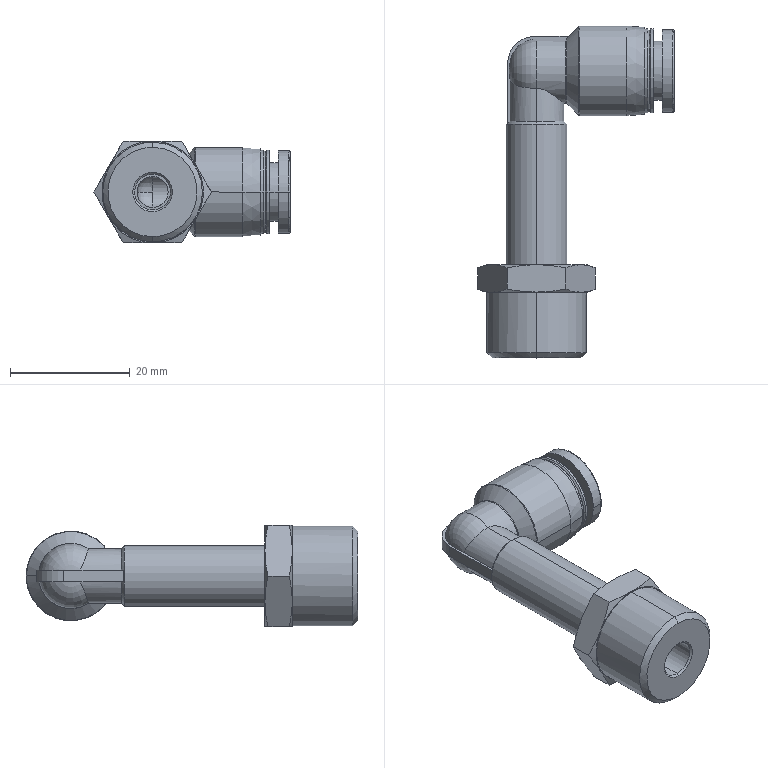Part | SolidWorks | features BaseBody 1 | 1 solid | 89 faces | box 32.815 x 55.5 x 17 mm | volume 7231 mm3 | cone 28 | cylinder 27 | plane 19 | torus 13 | sphere 2 | commonest cylinder face diameters 5.2 x4 14 x4 9.08 x3 6 x2 8 x2 9.9 x2